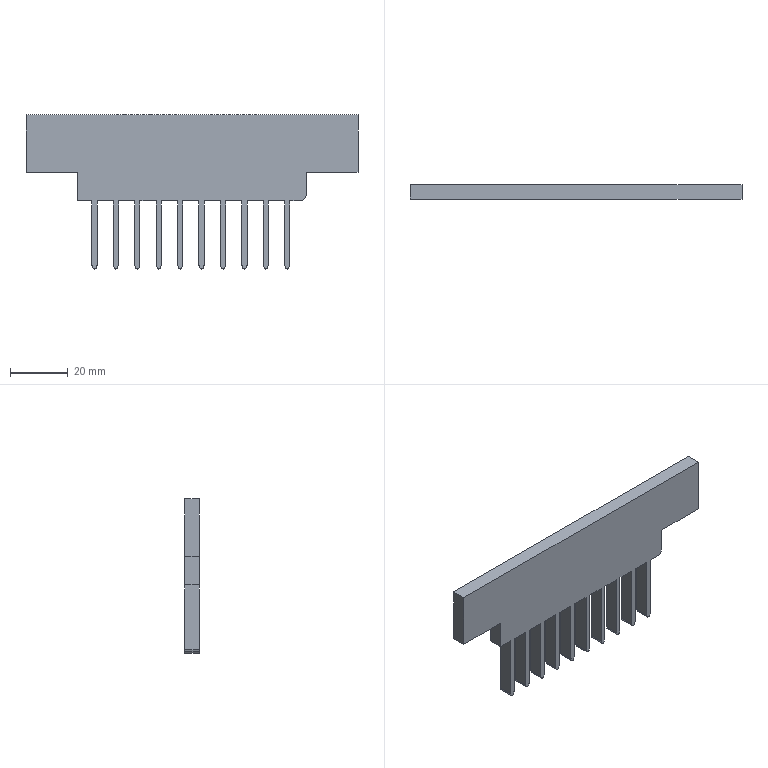Part | STEP file | 200 mesh_id2046 | 1 solid | 91 faces | box 115.071 x 4.98 x 53.4 mm | volume 17362 mm3 | plane 80 | cylinder 11 | commonest cylinder face diameters 1.211 x10 4 x1